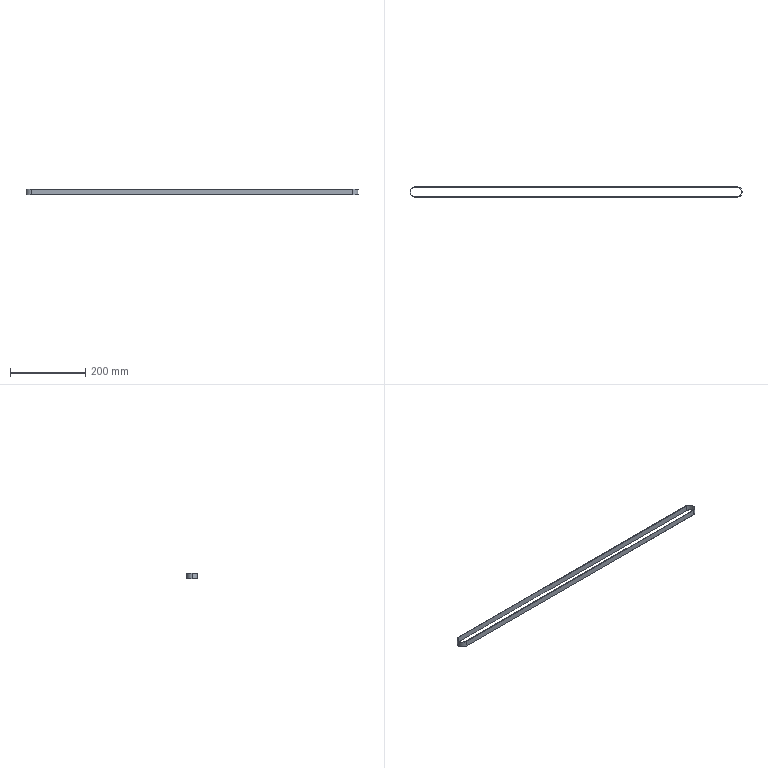Part | SolidWorks | features Extrusion 1 | 1 solid | 12 faces | box 880.84 x 28.34 x 15 mm | volume 31689 mm3 | cylinder 6 | plane 6 | commonest cylinder face diameters 25.98 x3 28.34 x3
STEP:
#1=CARTESIAN_POINT('',(0.,12.99,7.5));
#2=VERTEX_POINT('',#1);
#3=CARTESIAN_POINT('',(-12.99,0.,7.5));
#4=VERTEX_POINT('',#3);
#5=CARTESIAN_POINT('',(0.,0.,7.5));
#6=DIRECTION('',(0.,0.,1.));
#7=DIRECTION('',(1.,0.,0.));
#8=AXIS2_PLACEMENT_3D('',#5,#6,#7);
#9=CIRCLE('',#8,12.99);
#10=EDGE_CURVE('',#2,#4,#9,.T.);
#11=ORIENTED_EDGE('',*,*,#10,.T.);
#12=CARTESIAN_POINT('',(-12.99,0.,-7.5));
#13=VERTEX_POINT('',#12);
#14=CARTESIAN_POINT('',(-12.99,0.,7.5));
#15=DIRECTION('',(0.,0.,-1.));
#16=VECTOR('',#15,1000.);
#17=LINE('',#14,#16);
#18=EDGE_CURVE('',#4,#13,#17,.T.);
#19=ORIENTED_EDGE('',*,*,#18,.T.);
#20=CARTESIAN_POINT('',(0.,12.99,-7.5));
#21=VERTEX_POINT('',#20);
#22=CARTESIAN_POINT('',(0.,0.,-7.5));
#23=DIRECTION('',(0.,0.,1.));
#24=DIRECTION('',(1.,0.,0.));
#25=AXIS2_PLACEMENT_3D('',#22,#23,#24);
#26=CIRCLE('',#25,12.99);
#27=EDGE_CURVE('',#21,#13,#26,.T.);
#28=ORIENTED_EDGE('',*,*,#27,.F.);
#29=CARTESIAN_POINT('',(0.,12.99,7.5));
#30=DIRECTION('',(0.,0.,-1.));
#31=VECTOR('',#30,1000.);
#32=LINE('',#29,#31);
#33=EDGE_CURVE('',#2,#21,#32,.T.);
#34=ORIENTED_EDGE('',*,*,#33,.F.);
#35=EDGE_LOOP('',(#11,#19,#28,#34));
#36=FACE_OUTER_BOUND('',#35,.T.);
#37=CARTESIAN_POINT('',(0.,0.,7.5));
#38=DIRECTION('',(0.,0.,-1.));
#39=DIRECTION('',(-1.,0.,0.));
#40=AXIS2_PLACEMENT_3D('',#37,#38,#39);
#41=CYLINDRICAL_SURFACE('',#40,12.99);
#42=ADVANCED_FACE('',(#36),#41,.F.);
#43=CARTESIAN_POINT('',(-14.17,0.,7.5));
#44=VERTEX_POINT('',#43);
#45=CARTESIAN_POINT('',(0.,-14.17,7.5));
#46=VERTEX_POINT('',#45);
#47=CARTESIAN_POINT('',(0.,0.,7.5));
#48=DIRECTION('',(0.,0.,1.));
#49=DIRECTION('',(1.,0.,0.));
#50=AXIS2_PLACEMENT_3D('',#47,#48,#49);
#51=CIRCLE('',#50,14.17);
#52=EDGE_CURVE('',#44,#46,#51,.T.);
#53=ORIENTED_EDGE('',*,*,#52,.F.);
#54=CARTESIAN_POINT('',(-14.17,0.,-7.5));
#55=VERTEX_POINT('',#54);
#56=CARTESIAN_POINT('',(-14.17,0.,7.5));
#57=DIRECTION('',(0.,0.,-1.));
#58=VECTOR('',#57,1000.);
#59=LINE('',#56,#58);
#60=EDGE_CURVE('',#44,#55,#59,.T.);
#61=ORIENTED_EDGE('',*,*,#60,.T.);
#62=CARTESIAN_POINT('',(0.,-14.17,-7.5));
#63=VERTEX_POINT('',#62);
#64=CARTESIAN_POINT('',(0.,0.,-7.5));
#65=DIRECTION('',(0.,0.,1.));
#66=DIRECTION('',(1.,0.,0.));
#67=AXIS2_PLACEMENT_3D('',#64,#65,#66);
#68=CIRCLE('',#67,14.17);
#69=EDGE_CURVE('',#55,#63,#68,.T.);
#70=ORIENTED_EDGE('',*,*,#69,.T.);
#71=CARTESIAN_POINT('',(0.,-14.17,7.5));
#72=DIRECTION('',(0.,0.,-1.));
#73=VECTOR('',#72,1000.);
#74=LINE('',#71,#73);
#75=EDGE_CURVE('',#46,#63,#74,.T.);
#76=ORIENTED_EDGE('',*,*,#75,.F.);
#77=EDGE_LOOP('',(#53,#61,#70,#76));
#78=FACE_OUTER_BOUND('',#77,.T.);
#79=CARTESIAN_POINT('',(0.,0.,7.5));
#80=DIRECTION('',(0.,0.,-1.));
#81=DIRECTION('',(-1.,0.,0.));
#82=AXIS2_PLACEMENT_3D('',#79,#80,#81);
#83=CYLINDRICAL_SURFACE('',#82,14.17);
#84=ADVANCED_FACE('',(#78),#83,.T.);
#85=CARTESIAN_POINT('',(0.,14.17,7.5));
#86=VERTEX_POINT('',#85);
#87=CARTESIAN_POINT('',(0.,0.,7.5));
#88=DIRECTION('',(0.,0.,1.));
#89=DIRECTION('',(1.,0.,0.));
#90=AXIS2_PLACEMENT_3D('',#87,#88,#89);
#91=CIRCLE('',#90,14.17);
#92=EDGE_CURVE('',#86,#44,#91,.T.);
#93=ORIENTED_EDGE('',*,*,#92,.T.);
#94=ORIENTED_EDGE('',*,*,#52,.T.);
#95=CARTESIAN_POINT('',(852.5,-14.17,7.5));
#96=VERTEX_POINT('',#95);
#97=CARTESIAN_POINT('',(852.5,-14.17,7.5));
#98=DIRECTION('',(1.,0.,0.));
#99=VECTOR('',#98,1000.);
#100=LINE('',#97,#99);
#101=EDGE_CURVE('',#46,#96,#100,.T.);
#102=ORIENTED_EDGE('',*,*,#101,.T.);
#103=CARTESIAN_POINT('',(852.5,14.17,7.5));
#104=VERTEX_POINT('',#103);
#105=CARTESIAN_POINT('',(852.5,0.,7.5));
#106=DIRECTION('',(0.,0.,1.));
#107=DIRECTION('',(1.,0.,0.));
#108=AXIS2_PLACEMENT_3D('',#105,#106,#107);
#109=CIRCLE('',#108,14.17);
#110=EDGE_CURVE('',#96,#104,#109,.T.);
#111=ORIENTED_EDGE('',*,*,#110,.T.);
#112=CARTESIAN_POINT('',(0.,14.17,7.5));
#113=DIRECTION('',(-1.,0.,0.));
#114=VECTOR('',#113,1000.);
#115=LINE('',#112,#114);
#116=EDGE_CURVE('',#104,#86,#115,.T.);
#117=ORIENTED_EDGE('',*,*,#116,.T.);
#118=EDGE_LOOP('',(#93,#94,#102,#111,#117));
#119=FACE_OUTER_BOUND('',#118,.T.);
#120=CARTESIAN_POINT('',(0.,-12.99,7.5));
#121=VERTEX_POINT('',#120);
#122=CARTESIAN_POINT('',(852.5,-12.99,7.5));
#123=VERTEX_POINT('',#122);
#124=CARTESIAN_POINT('',(852.5,-12.99,7.5));
#125=DIRECTION('',(1.,0.,0.));
#126=VECTOR('',#125,1000.);
#127=LINE('',#124,#126);
#128=EDGE_CURVE('',#121,#123,#127,.T.);
#129=ORIENTED_EDGE('',*,*,#128,.F.);
#130=CARTESIAN_POINT('',(0.,0.,7.5));
#131=DIRECTION('',(0.,0.,1.));
#132=DIRECTION('',(1.,0.,0.));
#133=AXIS2_PLACEMENT_3D('',#130,#131,#132);
#134=CIRCLE('',#133,12.99);
#135=EDGE_CURVE('',#4,#121,#134,.T.);
#136=ORIENTED_EDGE('',*,*,#135,.F.);
#137=ORIENTED_EDGE('',*,*,#10,.F.);
#138=CARTESIAN_POINT('',(852.5,12.99,7.5));
#139=VERTEX_POINT('',#138);
#140=CARTESIAN_POINT('',(0.,12.99,7.5));
#141=DIRECTION('',(-1.,0.,0.));
#142=VECTOR('',#141,1000.);
#143=LINE('',#140,#142);
#144=EDGE_CURVE('',#139,#2,#143,.T.);
#145=ORIENTED_EDGE('',*,*,#144,.F.);
#146=CARTESIAN_POINT('',(852.5,0.,7.5));
#147=DIRECTION('',(0.,0.,1.));
#148=DIRECTION('',(1.,0.,0.));
#149=AXIS2_PLACEMENT_3D('',#146,#147,#148);
#150=CIRCLE('',#149,12.99);
#151=EDGE_CURVE('',#123,#139,#150,.T.);
#152=ORIENTED_EDGE('',*,*,#151,.F.);
#153=EDGE_LOOP('',(#129,#136,#137,#145,#152));
#154=FACE_BOUND('',#153,.T.);
#155=CARTESIAN_POINT('',(0.,0.,7.5));
#156=DIRECTION('',(0.,0.,1.));
#157=DIRECTION('',(1.,0.,0.));
#158=AXIS2_PLACEMENT_3D('',#155,#156,#157);
#159=PLANE('',#158);
#160=ADVANCED_FACE('',(#119,#154),#159,.T.);
#161=CARTESIAN_POINT('',(0.,14.17,-7.5));
#162=VERTEX_POINT('',#161);
#163=CARTESIAN_POINT('',(0.,0.,-7.5));
#164=DIRECTION('',(0.,0.,1.));
#165=DIRECTION('',(1.,0.,0.));
#166=AXIS2_PLACEMENT_3D('',#163,#164,#165);
#167=CIRCLE('',#166,14.17);
#168=EDGE_CURVE('',#162,#55,#167,.T.);
#169=ORIENTED_EDGE('',*,*,#168,.F.);
#170=CARTESIAN_POINT('',(852.5,14.17,-7.5));
#171=VERTEX_POINT('',#170);
#172=CARTESIAN_POINT('',(0.,14.17,-7.5));
#173=DIRECTION('',(-1.,0.,0.));
#174=VECTOR('',#173,1000.);
#175=LINE('',#172,#174);
#176=EDGE_CURVE('',#171,#162,#175,.T.);
#177=ORIENTED_EDGE('',*,*,#176,.F.);
#178=CARTESIAN_POINT('',(852.5,-14.17,-7.5));
#179=VERTEX_POINT('',#178);
#180=CARTESIAN_POINT('',(852.5,0.,-7.5));
#181=DIRECTION('',(0.,0.,1.));
#182=DIRECTION('',(1.,0.,0.));
#183=AXIS2_PLACEMENT_3D('',#180,#181,#182);
#184=CIRCLE('',#183,14.17);
#185=EDGE_CURVE('',#179,#171,#184,.T.);
#186=ORIENTED_EDGE('',*,*,#185,.F.);
#187=CARTESIAN_POINT('',(852.5,-14.17,-7.5));
#188=DIRECTION('',(1.,0.,0.));
#189=VECTOR('',#188,1000.);
#190=LINE('',#187,#189);
#191=EDGE_CURVE('',#63,#179,#190,.T.);
#192=ORIENTED_EDGE('',*,*,#191,.F.);
#193=ORIENTED_EDGE('',*,*,#69,.F.);
#194=EDGE_LOOP('',(#169,#177,#186,#192,#193));
#195=FACE_OUTER_BOUND('',#194,.T.);
#196=ORIENTED_EDGE('',*,*,#27,.T.);
#197=CARTESIAN_POINT('',(0.,-12.99,-7.5));
#198=VERTEX_POINT('',#197);
#199=CARTESIAN_POINT('',(0.,0.,-7.5));
#200=DIRECTION('',(0.,0.,1.));
#201=DIRECTION('',(1.,0.,0.));
#202=AXIS2_PLACEMENT_3D('',#199,#200,#201);
#203=CIRCLE('',#202,12.99);
#204=EDGE_CURVE('',#13,#198,#203,.T.);
#205=ORIENTED_EDGE('',*,*,#204,.T.);
#206=CARTESIAN_POINT('',(852.5,-12.99,-7.5));
#207=VERTEX_POINT('',#206);
#208=CARTESIAN_POINT('',(852.5,-12.99,-7.5));
#209=DIRECTION('',(1.,0.,0.));
#210=VECTOR('',#209,1000.);
#211=LINE('',#208,#210);
#212=EDGE_CURVE('',#198,#207,#211,.T.);
#213=ORIENTED_EDGE('',*,*,#212,.T.);
#214=CARTESIAN_POINT('',(852.5,12.99,-7.5));
#215=VERTEX_POINT('',#214);
#216=CARTESIAN_POINT('',(852.5,0.,-7.5));
#217=DIRECTION('',(0.,0.,1.));
#218=DIRECTION('',(1.,0.,0.));
#219=AXIS2_PLACEMENT_3D('',#216,#217,#218);
#220=CIRCLE('',#219,12.99);
#221=EDGE_CURVE('',#207,#215,#220,.T.);
#222=ORIENTED_EDGE('',*,*,#221,.T.);
#223=CARTESIAN_POINT('',(0.,12.99,-7.5));
#224=DIRECTION('',(-1.,0.,0.));
#225=VECTOR('',#224,1000.);
#226=LINE('',#223,#225);
#227=EDGE_CURVE('',#215,#21,#226,.T.);
#228=ORIENTED_EDGE('',*,*,#227,.T.);
#229=EDGE_LOOP('',(#196,#205,#213,#222,#228));
#230=FACE_BOUND('',#229,.T.);
#231=CARTESIAN_POINT('',(0.,0.,-7.5));
#232=DIRECTION('',(0.,0.,1.));
#233=DIRECTION('',(1.,0.,0.));
#234=AXIS2_PLACEMENT_3D('',#231,#232,#233);
#235=PLANE('',#234);
#236=ADVANCED_FACE('',(#195,#230),#235,.F.);
#237=ORIENTED_EDGE('',*,*,#60,.F.);
#238=ORIENTED_EDGE('',*,*,#92,.F.);
#239=CARTESIAN_POINT('',(0.,14.17,7.5));
#240=DIRECTION('',(0.,0.,-1.));
#241=VECTOR('',#240,1000.);
#242=LINE('',#239,#241);
#243=EDGE_CURVE('',#86,#162,#242,.T.);
#244=ORIENTED_EDGE('',*,*,#243,.T.);
#245=ORIENTED_EDGE('',*,*,#168,.T.);
#246=EDGE_LOOP('',(#237,#238,#244,#245));
#247=FACE_OUTER_BOUND('',#246,.T.);
#248=CARTESIAN_POINT('',(0.,0.,7.5));
#249=DIRECTION('',(0.,0.,-1.));
#250=DIRECTION('',(-1.,0.,0.));
#251=AXIS2_PLACEMENT_3D('',#248,#249,#250);
#252=CYLINDRICAL_SURFACE('',#251,14.17);
#253=ADVANCED_FACE('',(#247),#252,.T.);
#254=ORIENTED_EDGE('',*,*,#191,.T.);
#255=CARTESIAN_POINT('',(852.5,-14.17,7.5));
#256=DIRECTION('',(0.,0.,-1.));
#257=VECTOR('',#256,1000.);
#258=LINE('',#255,#257);
#259=EDGE_CURVE('',#96,#179,#258,.T.);
#260=ORIENTED_EDGE('',*,*,#259,.F.);
#261=ORIENTED_EDGE('',*,*,#101,.F.);
#262=ORIENTED_EDGE('',*,*,#75,.T.);
#263=EDGE_LOOP('',(#254,#260,#261,#262));
#264=FACE_OUTER_BOUND('',#263,.T.);
#265=CARTESIAN_POINT('',(852.5,-14.17,7.5));
#266=DIRECTION('',(0.,1.,0.));
#267=DIRECTION('',(0.,0.,1.));
#268=AXIS2_PLACEMENT_3D('',#265,#266,#267);
#269=PLANE('',#268);
#270=ADVANCED_FACE('',(#264),#269,.F.);
#271=ORIENTED_EDGE('',*,*,#185,.T.);
#272=CARTESIAN_POINT('',(852.5,14.17,7.5));
#273=DIRECTION('',(0.,0.,-1.));
#274=VECTOR('',#273,1000.);
#275=LINE('',#272,#274);
#276=EDGE_CURVE('',#104,#171,#275,.T.);
#277=ORIENTED_EDGE('',*,*,#276,.F.);
#278=ORIENTED_EDGE('',*,*,#110,.F.);
#279=ORIENTED_EDGE('',*,*,#259,.T.);
#280=EDGE_LOOP('',(#271,#277,#278,#279));
#281=FACE_OUTER_BOUND('',#280,.T.);
#282=CARTESIAN_POINT('',(852.5,0.,7.5));
#283=DIRECTION('',(0.,0.,-1.));
#284=DIRECTION('',(-1.,0.,0.));
#285=AXIS2_PLACEMENT_3D('',#282,#283,#284);
#286=CYLINDRICAL_SURFACE('',#285,14.17);
#287=ADVANCED_FACE('',(#281),#286,.T.);
#288=ORIENTED_EDGE('',*,*,#176,.T.);
#289=ORIENTED_EDGE('',*,*,#243,.F.);
#290=ORIENTED_EDGE('',*,*,#116,.F.);
#291=ORIENTED_EDGE('',*,*,#276,.T.);
#292=EDGE_LOOP('',(#288,#289,#290,#291));
#293=FACE_OUTER_BOUND('',#292,.T.);
#294=CARTESIAN_POINT('',(0.,14.17,7.5));
#295=DIRECTION('',(0.,-1.,0.));
#296=DIRECTION('',(0.,0.,-1.));
#297=AXIS2_PLACEMENT_3D('',#294,#295,#296);
#298=PLANE('',#297);
#299=ADVANCED_FACE('',(#293),#298,.F.);
#300=ORIENTED_EDGE('',*,*,#18,.F.);
#301=ORIENTED_EDGE('',*,*,#135,.T.);
#302=CARTESIAN_POINT('',(0.,-12.99,7.5));
#303=DIRECTION('',(0.,0.,-1.));
#304=VECTOR('',#303,1000.);
#305=LINE('',#302,#304);
#306=EDGE_CURVE('',#121,#198,#305,.T.);
#307=ORIENTED_EDGE('',*,*,#306,.T.);
#308=ORIENTED_EDGE('',*,*,#204,.F.);
#309=EDGE_LOOP('',(#300,#301,#307,#308));
#310=FACE_OUTER_BOUND('',#309,.T.);
#311=CARTESIAN_POINT('',(0.,0.,7.5));
#312=DIRECTION('',(0.,0.,-1.));
#313=DIRECTION('',(-1.,0.,0.));
#314=AXIS2_PLACEMENT_3D('',#311,#312,#313);
#315=CYLINDRICAL_SURFACE('',#314,12.99);
#316=ADVANCED_FACE('',(#310),#315,.F.);
#317=ORIENTED_EDGE('',*,*,#212,.F.);
#318=ORIENTED_EDGE('',*,*,#306,.F.);
#319=ORIENTED_EDGE('',*,*,#128,.T.);
#320=CARTESIAN_POINT('',(852.5,-12.99,7.5));
#321=DIRECTION('',(0.,0.,-1.));
#322=VECTOR('',#321,1000.);
#323=LINE('',#320,#322);
#324=EDGE_CURVE('',#123,#207,#323,.T.);
#325=ORIENTED_EDGE('',*,*,#324,.T.);
#326=EDGE_LOOP('',(#317,#318,#319,#325));
#327=FACE_OUTER_BOUND('',#326,.T.);
#328=CARTESIAN_POINT('',(852.5,-12.99,7.5));
#329=DIRECTION('',(0.,1.,0.));
#330=DIRECTION('',(0.,0.,1.));
#331=AXIS2_PLACEMENT_3D('',#328,#329,#330);
#332=PLANE('',#331);
#333=ADVANCED_FACE('',(#327),#332,.T.);
#334=ORIENTED_EDGE('',*,*,#221,.F.);
#335=ORIENTED_EDGE('',*,*,#324,.F.);
#336=ORIENTED_EDGE('',*,*,#151,.T.);
#337=CARTESIAN_POINT('',(852.5,12.99,7.5));
#338=DIRECTION('',(0.,0.,-1.));
#339=VECTOR('',#338,1000.);
#340=LINE('',#337,#339);
#341=EDGE_CURVE('',#139,#215,#340,.T.);
#342=ORIENTED_EDGE('',*,*,#341,.T.);
#343=EDGE_LOOP('',(#334,#335,#336,#342));
#344=FACE_OUTER_BOUND('',#343,.T.);
#345=CARTESIAN_POINT('',(852.5,0.,7.5));
#346=DIRECTION('',(0.,0.,-1.));
#347=DIRECTION('',(-1.,0.,0.));
#348=AXIS2_PLACEMENT_3D('',#345,#346,#347);
#349=CYLINDRICAL_SURFACE('',#348,12.99);
#350=ADVANCED_FACE('',(#344),#349,.F.);
#351=ORIENTED_EDGE('',*,*,#227,.F.);
#352=ORIENTED_EDGE('',*,*,#341,.F.);
#353=ORIENTED_EDGE('',*,*,#144,.T.);
#354=ORIENTED_EDGE('',*,*,#33,.T.);
#355=EDGE_LOOP('',(#351,#352,#353,#354));
#356=FACE_OUTER_BOUND('',#355,.T.);
#357=CARTESIAN_POINT('',(0.,12.99,7.5));
#358=DIRECTION('',(0.,-1.,0.));
#359=DIRECTION('',(0.,0.,-1.));
#360=AXIS2_PLACEMENT_3D('',#357,#358,#359);
#361=PLANE('',#360);
#362=ADVANCED_FACE('',(#356),#361,.T.);
#363=CLOSED_SHELL('',(#42,#84,#160,#236,#253,#270,#287,#299,#316,#333,#350,#362));
#364=MANIFOLD_SOLID_BREP('',#363);
#365=CARTESIAN_POINT('',(0.,0.,0.));
#366=DIRECTION('',(0.,0.,1.));
#367=DIRECTION('',(1.,0.,0.));
#368=AXIS2_PLACEMENT_3D('',#365,#366,#367);
#369=(LENGTH_UNIT()NAMED_UNIT(*)SI_UNIT(.MILLI.,.METRE.));
#370=UNCERTAINTY_MEASURE_WITH_UNIT(LENGTH_MEASURE(0.00001),#369,'','');
#371=(NAMED_UNIT(*)PLANE_ANGLE_UNIT()SI_UNIT($,.RADIAN.));
#372=(NAMED_UNIT(*)SI_UNIT($,.STERADIAN.)SOLID_ANGLE_UNIT());
#373=(GEOMETRIC_REPRESENTATION_CONTEXT(3)GLOBAL_UNCERTAINTY_ASSIGNED_CONTEXT((#370))GLOBAL_UNIT_ASSIGNED_CONTEXT((#369,#371,#372))REPRESENTATION_CONTEXT('',''));
#374=ADVANCED_BREP_SHAPE_REPRESENTATION('',(#364,#368),#373);